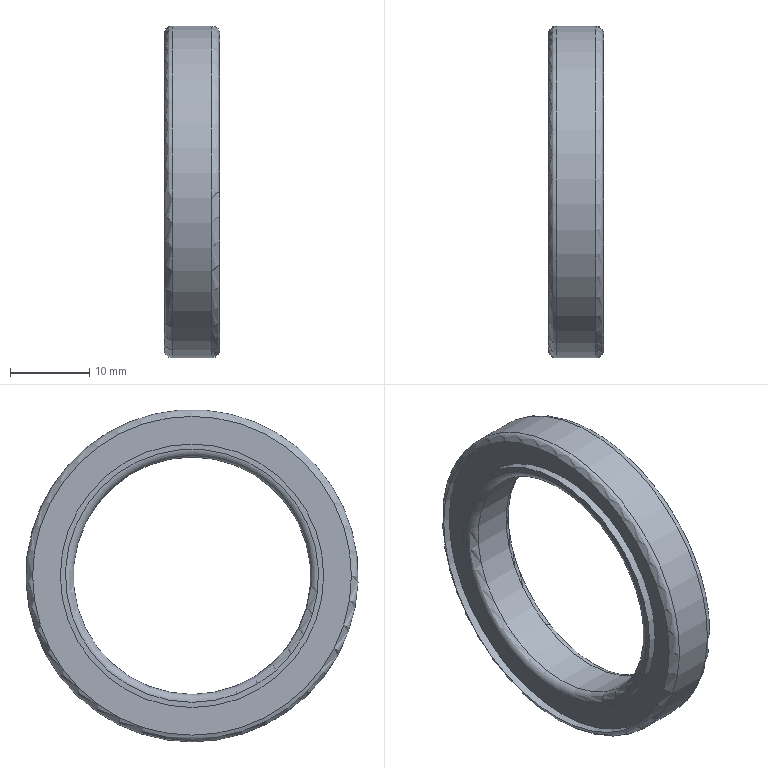Part | STEP file | GB276-1994 bearing 61806-2Z | 1 solid | 14 faces | box 7 x 42 x 42 mm | volume 3844 mm3 | cylinder 6 | plane 4 | torus 4 | commonest cylinder face diameters 33.3 x2 40.3 x2 30 x1 42 x1
STEP:
#1=CARTESIAN_POINT('',(-3.5,0.,-16.));
#2=VERTEX_POINT('',#1);
#3=CARTESIAN_POINT('',(-3.5,0.,0.));
#4=DIRECTION('',(1.,0.,0.));
#5=DIRECTION('',(0.,0.,-1.));
#6=AXIS2_PLACEMENT_3D('',#3,#4,#5);
#7=CIRCLE('',#6,16.);
#8=EDGE_CURVE('',#2,#2,#7,.T.);
#9=ORIENTED_EDGE('',*,*,#8,.T.);
#10=EDGE_LOOP('',(#9));
#11=FACE_BOUND('',#10,.T.);
#12=CARTESIAN_POINT('',(-3.5,0.,16.65));
#13=VERTEX_POINT('',#12);
#14=CARTESIAN_POINT('',(-3.5,0.,0.));
#15=DIRECTION('',(-1.,0.,0.));
#16=DIRECTION('',(0.,0.,1.));
#17=AXIS2_PLACEMENT_3D('',#14,#15,#16);
#18=CIRCLE('',#17,16.65);
#19=EDGE_CURVE('',#13,#13,#18,.T.);
#20=ORIENTED_EDGE('',*,*,#19,.T.);
#21=EDGE_LOOP('',(#20));
#22=FACE_OUTER_BOUND('',#21,.T.);
#23=CARTESIAN_POINT('',(-3.5,0.,0.));
#24=DIRECTION('',(1.,0.,0.));
#25=DIRECTION('',(0.,0.,-1.));
#26=AXIS2_PLACEMENT_3D('',#23,#24,#25);
#27=PLANE('',#26);
#28=ADVANCED_FACE('',(#11,#22),#27,.F.);
#29=CARTESIAN_POINT('',(3.5,0.,-16.));
#30=VERTEX_POINT('',#29);
#31=CARTESIAN_POINT('',(3.5,0.,0.));
#32=DIRECTION('',(-1.,0.,0.));
#33=DIRECTION('',(0.,0.,-1.));
#34=AXIS2_PLACEMENT_3D('',#31,#32,#33);
#35=CIRCLE('',#34,16.);
#36=EDGE_CURVE('',#30,#30,#35,.T.);
#37=ORIENTED_EDGE('',*,*,#36,.T.);
#38=EDGE_LOOP('',(#37));
#39=FACE_BOUND('',#38,.T.);
#40=CARTESIAN_POINT('',(3.5,0.,-16.65));
#41=VERTEX_POINT('',#40);
#42=CARTESIAN_POINT('',(3.5,0.,0.));
#43=DIRECTION('',(1.,0.,0.));
#44=DIRECTION('',(0.,0.,-1.));
#45=AXIS2_PLACEMENT_3D('',#42,#43,#44);
#46=CIRCLE('',#45,16.65);
#47=EDGE_CURVE('',#41,#41,#46,.T.);
#48=ORIENTED_EDGE('',*,*,#47,.T.);
#49=EDGE_LOOP('',(#48));
#50=FACE_OUTER_BOUND('',#49,.T.);
#51=CARTESIAN_POINT('',(3.5,0.,0.));
#52=DIRECTION('',(1.,0.,0.));
#53=DIRECTION('',(0.,0.,-1.));
#54=AXIS2_PLACEMENT_3D('',#51,#52,#53);
#55=PLANE('',#54);
#56=ADVANCED_FACE('',(#39,#50),#55,.T.);
#57=CARTESIAN_POINT('',(-2.5,0.,-21.));
#58=VERTEX_POINT('',#57);
#59=CARTESIAN_POINT('',(-2.5,0.,0.));
#60=DIRECTION('',(1.,0.,0.));
#61=DIRECTION('',(0.,0.,-1.));
#62=AXIS2_PLACEMENT_3D('',#59,#60,#61);
#63=CIRCLE('',#62,21.);
#64=EDGE_CURVE('',#58,#58,#63,.T.);
#65=ORIENTED_EDGE('',*,*,#64,.T.);
#66=EDGE_LOOP('',(#65));
#67=FACE_OUTER_BOUND('',#66,.T.);
#68=CARTESIAN_POINT('',(2.5,0.,-21.));
#69=VERTEX_POINT('',#68);
#70=CARTESIAN_POINT('',(2.5,0.,0.));
#71=DIRECTION('',(-1.,0.,0.));
#72=DIRECTION('',(0.,0.,-1.));
#73=AXIS2_PLACEMENT_3D('',#70,#71,#72);
#74=CIRCLE('',#73,21.);
#75=EDGE_CURVE('',#69,#69,#74,.T.);
#76=ORIENTED_EDGE('',*,*,#75,.T.);
#77=EDGE_LOOP('',(#76));
#78=FACE_OUTER_BOUND('',#77,.T.);
#79=CARTESIAN_POINT('',(3.5,0.,0.));
#80=DIRECTION('',(-1.,0.,0.));
#81=DIRECTION('',(0.,0.,1.));
#82=AXIS2_PLACEMENT_3D('',#79,#80,#81);
#83=CYLINDRICAL_SURFACE('',#82,21.);
#84=ADVANCED_FACE('',(#67,#78),#83,.T.);
#85=CARTESIAN_POINT('',(-2.5,0.,-15.));
#86=VERTEX_POINT('',#85);
#87=CARTESIAN_POINT('',(-2.5,0.,0.));
#88=DIRECTION('',(-1.,0.,0.));
#89=DIRECTION('',(0.,0.,-1.));
#90=AXIS2_PLACEMENT_3D('',#87,#88,#89);
#91=CIRCLE('',#90,15.);
#92=EDGE_CURVE('',#86,#86,#91,.T.);
#93=ORIENTED_EDGE('',*,*,#92,.T.);
#94=EDGE_LOOP('',(#93));
#95=FACE_OUTER_BOUND('',#94,.T.);
#96=CARTESIAN_POINT('',(2.5,0.,-15.));
#97=VERTEX_POINT('',#96);
#98=CARTESIAN_POINT('',(2.5,0.,0.));
#99=DIRECTION('',(1.,0.,0.));
#100=DIRECTION('',(0.,0.,-1.));
#101=AXIS2_PLACEMENT_3D('',#98,#99,#100);
#102=CIRCLE('',#101,15.);
#103=EDGE_CURVE('',#97,#97,#102,.T.);
#104=ORIENTED_EDGE('',*,*,#103,.T.);
#105=EDGE_LOOP('',(#104));
#106=FACE_OUTER_BOUND('',#105,.T.);
#107=CARTESIAN_POINT('',(3.5,0.,0.));
#108=DIRECTION('',(-1.,0.,0.));
#109=DIRECTION('',(0.,0.,1.));
#110=AXIS2_PLACEMENT_3D('',#107,#108,#109);
#111=CYLINDRICAL_SURFACE('',#110,15.);
#112=ADVANCED_FACE('',(#95,#106),#111,.F.);
#113=CARTESIAN_POINT('',(-3.489,0.,-20.15));
#114=VERTEX_POINT('',#113);
#115=CARTESIAN_POINT('',(-3.489,0.,0.));
#116=DIRECTION('',(-1.,0.,0.));
#117=DIRECTION('',(0.,0.,-1.));
#118=AXIS2_PLACEMENT_3D('',#115,#116,#117);
#119=CIRCLE('',#118,20.15);
#120=EDGE_CURVE('',#114,#114,#119,.T.);
#121=ORIENTED_EDGE('',*,*,#120,.F.);
#122=EDGE_LOOP('',(#121));
#123=FACE_OUTER_BOUND('',#122,.T.);
#124=ORIENTED_EDGE('',*,*,#64,.F.);
#125=EDGE_LOOP('',(#124));
#126=FACE_OUTER_BOUND('',#125,.T.);
#127=CARTESIAN_POINT('',(-2.5,0.,0.));
#128=DIRECTION('',(1.,0.,0.));
#129=DIRECTION('',(0.,0.,-1.));
#130=AXIS2_PLACEMENT_3D('',#127,#128,#129);
#131=TOROIDAL_SURFACE('',#130,20.,1.);
#132=ADVANCED_FACE('',(#123,#126),#131,.T.);
#133=CARTESIAN_POINT('',(3.489,0.,20.15));
#134=VERTEX_POINT('',#133);
#135=CARTESIAN_POINT('',(3.489,0.,0.));
#136=DIRECTION('',(1.,0.,0.));
#137=DIRECTION('',(0.,0.,1.));
#138=AXIS2_PLACEMENT_3D('',#135,#136,#137);
#139=CIRCLE('',#138,20.15);
#140=EDGE_CURVE('',#134,#134,#139,.T.);
#141=ORIENTED_EDGE('',*,*,#140,.F.);
#142=EDGE_LOOP('',(#141));
#143=FACE_OUTER_BOUND('',#142,.T.);
#144=ORIENTED_EDGE('',*,*,#75,.F.);
#145=EDGE_LOOP('',(#144));
#146=FACE_OUTER_BOUND('',#145,.T.);
#147=CARTESIAN_POINT('',(2.5,0.,0.));
#148=DIRECTION('',(1.,0.,0.));
#149=DIRECTION('',(0.,0.,-1.));
#150=AXIS2_PLACEMENT_3D('',#147,#148,#149);
#151=TOROIDAL_SURFACE('',#150,20.,1.);
#152=ADVANCED_FACE('',(#143,#146),#151,.T.);
#153=ORIENTED_EDGE('',*,*,#92,.F.);
#154=EDGE_LOOP('',(#153));
#155=FACE_OUTER_BOUND('',#154,.T.);
#156=ORIENTED_EDGE('',*,*,#8,.F.);
#157=EDGE_LOOP('',(#156));
#158=FACE_OUTER_BOUND('',#157,.T.);
#159=CARTESIAN_POINT('',(-2.5,0.,0.));
#160=DIRECTION('',(1.,0.,0.));
#161=DIRECTION('',(0.,0.,-1.));
#162=AXIS2_PLACEMENT_3D('',#159,#160,#161);
#163=TOROIDAL_SURFACE('',#162,16.,1.);
#164=ADVANCED_FACE('',(#155,#158),#163,.T.);
#165=ORIENTED_EDGE('',*,*,#36,.F.);
#166=EDGE_LOOP('',(#165));
#167=FACE_OUTER_BOUND('',#166,.T.);
#168=ORIENTED_EDGE('',*,*,#103,.F.);
#169=EDGE_LOOP('',(#168));
#170=FACE_OUTER_BOUND('',#169,.T.);
#171=CARTESIAN_POINT('',(2.5,0.,0.));
#172=DIRECTION('',(1.,0.,0.));
#173=DIRECTION('',(0.,0.,-1.));
#174=AXIS2_PLACEMENT_3D('',#171,#172,#173);
#175=TOROIDAL_SURFACE('',#174,16.,1.);
#176=ADVANCED_FACE('',(#167,#170),#175,.T.);
#177=ORIENTED_EDGE('',*,*,#140,.T.);
#178=EDGE_LOOP('',(#177));
#179=FACE_OUTER_BOUND('',#178,.T.);
#180=CARTESIAN_POINT('',(2.5,0.,-20.15));
#181=VERTEX_POINT('',#180);
#182=CARTESIAN_POINT('',(2.5,0.,0.));
#183=DIRECTION('',(1.,0.,0.));
#184=DIRECTION('',(0.,0.,-1.));
#185=AXIS2_PLACEMENT_3D('',#182,#183,#184);
#186=CIRCLE('',#185,20.15);
#187=EDGE_CURVE('',#181,#181,#186,.T.);
#188=ORIENTED_EDGE('',*,*,#187,.F.);
#189=EDGE_LOOP('',(#188));
#190=FACE_OUTER_BOUND('',#189,.T.);
#191=CARTESIAN_POINT('',(2.5,0.,0.));
#192=DIRECTION('',(1.,0.,0.));
#193=DIRECTION('',(0.,0.,-1.));
#194=AXIS2_PLACEMENT_3D('',#191,#192,#193);
#195=CYLINDRICAL_SURFACE('',#194,20.15);
#196=ADVANCED_FACE('',(#179,#190),#195,.F.);
#197=CARTESIAN_POINT('',(2.5,0.,-16.65));
#198=VERTEX_POINT('',#197);
#199=CARTESIAN_POINT('',(2.5,0.,0.));
#200=DIRECTION('',(1.,0.,0.));
#201=DIRECTION('',(0.,0.,-1.));
#202=AXIS2_PLACEMENT_3D('',#199,#200,#201);
#203=CIRCLE('',#202,16.65);
#204=EDGE_CURVE('',#198,#198,#203,.T.);
#205=ORIENTED_EDGE('',*,*,#204,.F.);
#206=EDGE_LOOP('',(#205));
#207=FACE_BOUND('',#206,.T.);
#208=ORIENTED_EDGE('',*,*,#187,.T.);
#209=EDGE_LOOP('',(#208));
#210=FACE_OUTER_BOUND('',#209,.T.);
#211=CARTESIAN_POINT('',(2.5,0.,0.));
#212=DIRECTION('',(1.,0.,0.));
#213=DIRECTION('',(0.,0.,-1.));
#214=AXIS2_PLACEMENT_3D('',#211,#212,#213);
#215=PLANE('',#214);
#216=ADVANCED_FACE('',(#207,#210),#215,.T.);
#217=ORIENTED_EDGE('',*,*,#204,.T.);
#218=EDGE_LOOP('',(#217));
#219=FACE_OUTER_BOUND('',#218,.T.);
#220=ORIENTED_EDGE('',*,*,#47,.F.);
#221=EDGE_LOOP('',(#220));
#222=FACE_OUTER_BOUND('',#221,.T.);
#223=CARTESIAN_POINT('',(2.5,0.,0.));
#224=DIRECTION('',(1.,0.,0.));
#225=DIRECTION('',(0.,0.,-1.));
#226=AXIS2_PLACEMENT_3D('',#223,#224,#225);
#227=CYLINDRICAL_SURFACE('',#226,16.65);
#228=ADVANCED_FACE('',(#219,#222),#227,.T.);
#229=ORIENTED_EDGE('',*,*,#120,.T.);
#230=EDGE_LOOP('',(#229));
#231=FACE_OUTER_BOUND('',#230,.T.);
#232=CARTESIAN_POINT('',(-2.5,0.,20.15));
#233=VERTEX_POINT('',#232);
#234=CARTESIAN_POINT('',(-2.5,0.,0.));
#235=DIRECTION('',(-1.,0.,0.));
#236=DIRECTION('',(0.,0.,1.));
#237=AXIS2_PLACEMENT_3D('',#234,#235,#236);
#238=CIRCLE('',#237,20.15);
#239=EDGE_CURVE('',#233,#233,#238,.T.);
#240=ORIENTED_EDGE('',*,*,#239,.F.);
#241=EDGE_LOOP('',(#240));
#242=FACE_OUTER_BOUND('',#241,.T.);
#243=CARTESIAN_POINT('',(-2.5,0.,0.));
#244=DIRECTION('',(-1.,0.,0.));
#245=DIRECTION('',(0.,0.,1.));
#246=AXIS2_PLACEMENT_3D('',#243,#244,#245);
#247=CYLINDRICAL_SURFACE('',#246,20.15);
#248=ADVANCED_FACE('',(#231,#242),#247,.F.);
#249=CARTESIAN_POINT('',(-2.5,0.,16.65));
#250=VERTEX_POINT('',#249);
#251=CARTESIAN_POINT('',(-2.5,0.,0.));
#252=DIRECTION('',(-1.,0.,0.));
#253=DIRECTION('',(0.,0.,1.));
#254=AXIS2_PLACEMENT_3D('',#251,#252,#253);
#255=CIRCLE('',#254,16.65);
#256=EDGE_CURVE('',#250,#250,#255,.T.);
#257=ORIENTED_EDGE('',*,*,#256,.F.);
#258=EDGE_LOOP('',(#257));
#259=FACE_BOUND('',#258,.T.);
#260=ORIENTED_EDGE('',*,*,#239,.T.);
#261=EDGE_LOOP('',(#260));
#262=FACE_OUTER_BOUND('',#261,.T.);
#263=CARTESIAN_POINT('',(-2.5,0.,0.));
#264=DIRECTION('',(-1.,0.,0.));
#265=DIRECTION('',(0.,0.,1.));
#266=AXIS2_PLACEMENT_3D('',#263,#264,#265);
#267=PLANE('',#266);
#268=ADVANCED_FACE('',(#259,#262),#267,.T.);
#269=ORIENTED_EDGE('',*,*,#256,.T.);
#270=EDGE_LOOP('',(#269));
#271=FACE_OUTER_BOUND('',#270,.T.);
#272=ORIENTED_EDGE('',*,*,#19,.F.);
#273=EDGE_LOOP('',(#272));
#274=FACE_OUTER_BOUND('',#273,.T.);
#275=CARTESIAN_POINT('',(-2.5,0.,0.));
#276=DIRECTION('',(-1.,0.,0.));
#277=DIRECTION('',(0.,0.,1.));
#278=AXIS2_PLACEMENT_3D('',#275,#276,#277);
#279=CYLINDRICAL_SURFACE('',#278,16.65);
#280=ADVANCED_FACE('',(#271,#274),#279,.T.);
#281=CLOSED_SHELL('',(#28,#56,#84,#112,#132,#152,#164,#176,#196,#216,#228,#248,#268,#280));
#282=MANIFOLD_SOLID_BREP('',#281);
#283=CARTESIAN_POINT('',(0.,0.,0.));
#284=DIRECTION('',(0.,0.,1.));
#285=DIRECTION('',(1.,0.,0.));
#286=AXIS2_PLACEMENT_3D('',#283,#284,#285);
#287=(LENGTH_UNIT()NAMED_UNIT(*)SI_UNIT(.MILLI.,.METRE.));
#288=UNCERTAINTY_MEASURE_WITH_UNIT(LENGTH_MEASURE(0.00001),#287,'','');
#289=(NAMED_UNIT(*)PLANE_ANGLE_UNIT()SI_UNIT($,.RADIAN.));
#290=(NAMED_UNIT(*)SI_UNIT($,.STERADIAN.)SOLID_ANGLE_UNIT());
#291=(GEOMETRIC_REPRESENTATION_CONTEXT(3)GLOBAL_UNCERTAINTY_ASSIGNED_CONTEXT((#288))GLOBAL_UNIT_ASSIGNED_CONTEXT((#287,#289,#290))REPRESENTATION_CONTEXT('',''));
#292=ADVANCED_BREP_SHAPE_REPRESENTATION('',(#282,#286),#291);